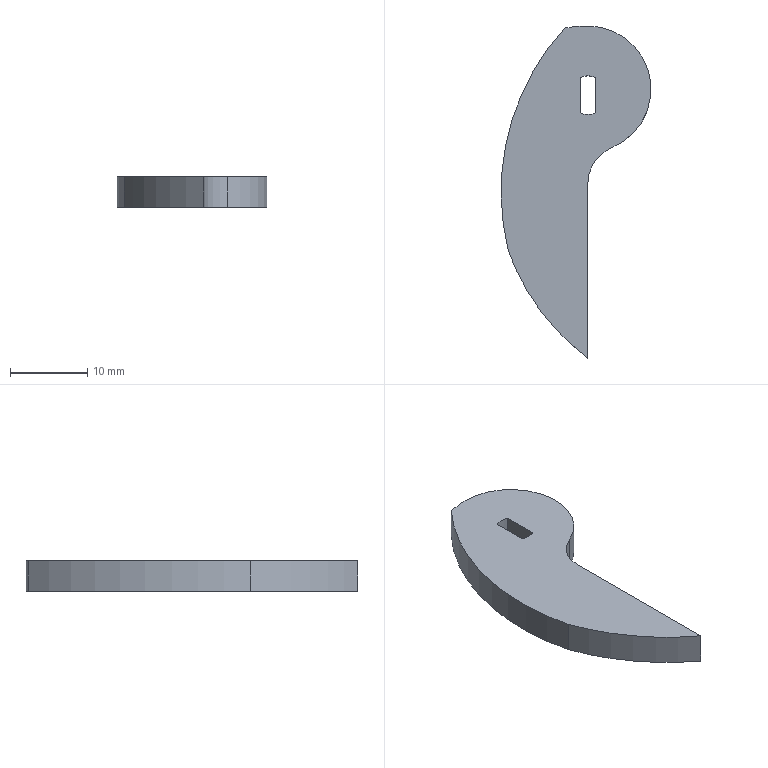Part | SolidWorks | features ICE 4, MirrorStock 1 | 1 solid | 12 faces | box 19.397 x 42.95 x 4 mm | volume 1803 mm3 | cylinder 7 | plane 5 | commonest cylinder face diameters 5 x2 10 x1 16.35 x1 32.7 x1 59.676 x1 62.992 x1
STEP:
#1=CARTESIAN_POINT('',(1.,0.9587,-4.));
#2=VERTEX_POINT('',#1);
#3=CARTESIAN_POINT('',(-1.,0.9587,-4.));
#4=VERTEX_POINT('',#3);
#5=CARTESIAN_POINT('',(0.,3.25,-4.));
#6=DIRECTION('',(0.,0.,-1.));
#7=DIRECTION('',(-1.,0.,0.));
#8=AXIS2_PLACEMENT_3D('',#5,#6,#7);
#9=CIRCLE('',#8,2.5);
#10=EDGE_CURVE('',#2,#4,#9,.T.);
#11=ORIENTED_EDGE('',*,*,#10,.F.);
#12=CARTESIAN_POINT('',(1.,5.541,-4.));
#13=VERTEX_POINT('',#12);
#14=CARTESIAN_POINT('',(1.,4.025,-4.));
#15=DIRECTION('',(0.,-1.,0.));
#16=VECTOR('',#15,1000.);
#17=LINE('',#14,#16);
#18=EDGE_CURVE('',#13,#2,#17,.T.);
#19=ORIENTED_EDGE('',*,*,#18,.F.);
#20=CARTESIAN_POINT('',(-1.,5.541,-4.));
#21=VERTEX_POINT('',#20);
#22=CARTESIAN_POINT('',(0.,3.25,-4.));
#23=DIRECTION('',(0.,0.,-1.));
#24=DIRECTION('',(-1.,0.,0.));
#25=AXIS2_PLACEMENT_3D('',#22,#23,#24);
#26=CIRCLE('',#25,2.5);
#27=EDGE_CURVE('',#21,#13,#26,.T.);
#28=ORIENTED_EDGE('',*,*,#27,.F.);
#29=CARTESIAN_POINT('',(-1.,4.025,-4.));
#30=DIRECTION('',(0.,1.,0.));
#31=VECTOR('',#30,1000.);
#32=LINE('',#29,#31);
#33=EDGE_CURVE('',#4,#21,#32,.T.);
#34=ORIENTED_EDGE('',*,*,#33,.F.);
#35=EDGE_LOOP('',(#11,#19,#28,#34));
#36=FACE_BOUND('',#35,.T.);
#37=CARTESIAN_POINT('',(-3.009,11.921,-4.));
#38=VERTEX_POINT('',#37);
#39=CARTESIAN_POINT('',(-10.302,-16.846,-4.));
#40=VERTEX_POINT('',#39);
#41=CARTESIAN_POINT('',(20.274,-9.29,-4.));
#42=DIRECTION('',(0.,0.,1.));
#43=DIRECTION('',(-1.,0.,0.));
#44=AXIS2_PLACEMENT_3D('',#41,#42,#43);
#45=CIRCLE('',#44,31.496);
#46=EDGE_CURVE('',#38,#40,#45,.T.);
#47=ORIENTED_EDGE('',*,*,#46,.F.);
#48=CARTESIAN_POINT('',(0.,12.2,-4.));
#49=VERTEX_POINT('',#48);
#50=CARTESIAN_POINT('',(0.,-4.15,-4.));
#51=DIRECTION('',(0.,0.,1.));
#52=DIRECTION('',(1.,0.,0.));
#53=AXIS2_PLACEMENT_3D('',#50,#51,#52);
#54=CIRCLE('',#53,16.35);
#55=EDGE_CURVE('',#49,#38,#54,.T.);
#56=ORIENTED_EDGE('',*,*,#55,.F.);
#57=CARTESIAN_POINT('',(3.102,-3.538,-4.));
#58=VERTEX_POINT('',#57);
#59=CARTESIAN_POINT('',(0.,4.025,-4.));
#60=DIRECTION('',(0.,0.,1.));
#61=DIRECTION('',(1.,0.,0.));
#62=AXIS2_PLACEMENT_3D('',#59,#60,#61);
#63=CIRCLE('',#62,8.175);
#64=EDGE_CURVE('',#58,#49,#63,.T.);
#65=ORIENTED_EDGE('',*,*,#64,.F.);
#66=CARTESIAN_POINT('',(0.,-8.164,-4.));
#67=VERTEX_POINT('',#66);
#68=CARTESIAN_POINT('',(5.,-8.164,-4.));
#69=DIRECTION('',(0.,0.,1.));
#70=DIRECTION('',(1.,0.,0.));
#71=AXIS2_PLACEMENT_3D('',#68,#69,#70);
#72=CIRCLE('',#71,5.);
#73=EDGE_CURVE('',#58,#67,#72,.T.);
#74=ORIENTED_EDGE('',*,*,#73,.T.);
#75=CARTESIAN_POINT('',(0.,-30.75,-4.));
#76=VERTEX_POINT('',#75);
#77=CARTESIAN_POINT('',(0.,-20.5,-4.));
#78=DIRECTION('',(0.,1.,0.));
#79=VECTOR('',#78,1000.);
#80=LINE('',#77,#79);
#81=EDGE_CURVE('',#76,#67,#80,.T.);
#82=ORIENTED_EDGE('',*,*,#81,.F.);
#83=CARTESIAN_POINT('',(17.793,-6.798,-4.));
#84=DIRECTION('',(0.,0.,-1.));
#85=DIRECTION('',(-1.,0.,0.));
#86=AXIS2_PLACEMENT_3D('',#83,#84,#85);
#87=CIRCLE('',#86,29.838);
#88=EDGE_CURVE('',#76,#40,#87,.T.);
#89=ORIENTED_EDGE('',*,*,#88,.T.);
#90=EDGE_LOOP('',(#47,#56,#65,#74,#82,#89));
#91=FACE_OUTER_BOUND('',#90,.T.);
#92=CARTESIAN_POINT('',(0.,4.025,-4.));
#93=DIRECTION('',(0.,0.,-1.));
#94=DIRECTION('',(1.,0.,0.));
#95=AXIS2_PLACEMENT_3D('',#92,#93,#94);
#96=PLANE('',#95);
#97=ADVANCED_FACE('',(#36,#91),#96,.T.);
#98=CARTESIAN_POINT('',(1.,0.9587,0.));
#99=VERTEX_POINT('',#98);
#100=CARTESIAN_POINT('',(1.,5.541,0.));
#101=VERTEX_POINT('',#100);
#102=CARTESIAN_POINT('',(1.,5.541,0.));
#103=DIRECTION('',(0.,1.,0.));
#104=VECTOR('',#103,1000.);
#105=LINE('',#102,#104);
#106=EDGE_CURVE('',#99,#101,#105,.T.);
#107=ORIENTED_EDGE('',*,*,#106,.F.);
#108=CARTESIAN_POINT('',(-1.,0.9587,0.));
#109=VERTEX_POINT('',#108);
#110=CARTESIAN_POINT('',(0.,3.25,0.));
#111=DIRECTION('',(0.,0.,1.));
#112=DIRECTION('',(1.,0.,0.));
#113=AXIS2_PLACEMENT_3D('',#110,#111,#112);
#114=CIRCLE('',#113,2.5);
#115=EDGE_CURVE('',#109,#99,#114,.T.);
#116=ORIENTED_EDGE('',*,*,#115,.F.);
#117=CARTESIAN_POINT('',(-1.,5.541,0.));
#118=VERTEX_POINT('',#117);
#119=CARTESIAN_POINT('',(-1.,5.541,0.));
#120=DIRECTION('',(0.,-1.,0.));
#121=VECTOR('',#120,1000.);
#122=LINE('',#119,#121);
#123=EDGE_CURVE('',#118,#109,#122,.T.);
#124=ORIENTED_EDGE('',*,*,#123,.F.);
#125=CARTESIAN_POINT('',(0.,3.25,0.));
#126=DIRECTION('',(0.,0.,1.));
#127=DIRECTION('',(1.,0.,0.));
#128=AXIS2_PLACEMENT_3D('',#125,#126,#127);
#129=CIRCLE('',#128,2.5);
#130=EDGE_CURVE('',#101,#118,#129,.T.);
#131=ORIENTED_EDGE('',*,*,#130,.F.);
#132=EDGE_LOOP('',(#107,#116,#124,#131));
#133=FACE_BOUND('',#132,.T.);
#134=CARTESIAN_POINT('',(0.,12.2,0.));
#135=VERTEX_POINT('',#134);
#136=CARTESIAN_POINT('',(-3.009,11.921,0.));
#137=VERTEX_POINT('',#136);
#138=CARTESIAN_POINT('',(0.,-4.15,0.));
#139=DIRECTION('',(0.,0.,1.));
#140=DIRECTION('',(1.,0.,0.));
#141=AXIS2_PLACEMENT_3D('',#138,#139,#140);
#142=CIRCLE('',#141,16.35);
#143=EDGE_CURVE('',#135,#137,#142,.T.);
#144=ORIENTED_EDGE('',*,*,#143,.T.);
#145=CARTESIAN_POINT('',(-10.302,-16.846,0.));
#146=VERTEX_POINT('',#145);
#147=CARTESIAN_POINT('',(20.274,-9.29,0.));
#148=DIRECTION('',(0.,0.,-1.));
#149=DIRECTION('',(-1.,0.,0.));
#150=AXIS2_PLACEMENT_3D('',#147,#148,#149);
#151=CIRCLE('',#150,31.496);
#152=EDGE_CURVE('',#146,#137,#151,.T.);
#153=ORIENTED_EDGE('',*,*,#152,.F.);
#154=CARTESIAN_POINT('',(0.,-30.75,0.));
#155=VERTEX_POINT('',#154);
#156=CARTESIAN_POINT('',(17.793,-6.798,0.));
#157=DIRECTION('',(0.,0.,-1.));
#158=DIRECTION('',(1.,0.,0.));
#159=AXIS2_PLACEMENT_3D('',#156,#157,#158);
#160=CIRCLE('',#159,29.838);
#161=EDGE_CURVE('',#155,#146,#160,.T.);
#162=ORIENTED_EDGE('',*,*,#161,.F.);
#163=CARTESIAN_POINT('',(0.,-8.164,0.));
#164=VERTEX_POINT('',#163);
#165=CARTESIAN_POINT('',(0.,-20.5,0.));
#166=DIRECTION('',(0.,1.,0.));
#167=VECTOR('',#166,1000.);
#168=LINE('',#165,#167);
#169=EDGE_CURVE('',#155,#164,#168,.T.);
#170=ORIENTED_EDGE('',*,*,#169,.T.);
#171=CARTESIAN_POINT('',(3.102,-3.538,0.));
#172=VERTEX_POINT('',#171);
#173=CARTESIAN_POINT('',(5.,-8.164,0.));
#174=DIRECTION('',(0.,0.,-1.));
#175=DIRECTION('',(1.,0.,0.));
#176=AXIS2_PLACEMENT_3D('',#173,#174,#175);
#177=CIRCLE('',#176,5.);
#178=EDGE_CURVE('',#164,#172,#177,.T.);
#179=ORIENTED_EDGE('',*,*,#178,.T.);
#180=CARTESIAN_POINT('',(0.,4.025,0.));
#181=DIRECTION('',(0.,0.,1.));
#182=DIRECTION('',(1.,0.,0.));
#183=AXIS2_PLACEMENT_3D('',#180,#181,#182);
#184=CIRCLE('',#183,8.175);
#185=EDGE_CURVE('',#172,#135,#184,.T.);
#186=ORIENTED_EDGE('',*,*,#185,.T.);
#187=EDGE_LOOP('',(#144,#153,#162,#170,#179,#186));
#188=FACE_OUTER_BOUND('',#187,.T.);
#189=CARTESIAN_POINT('',(0.,4.025,0.));
#190=DIRECTION('',(0.,0.,-1.));
#191=DIRECTION('',(1.,0.,0.));
#192=AXIS2_PLACEMENT_3D('',#189,#190,#191);
#193=PLANE('',#192);
#194=ADVANCED_FACE('',(#133,#188),#193,.F.);
#195=ORIENTED_EDGE('',*,*,#55,.T.);
#196=CARTESIAN_POINT('',(-3.009,11.921,-10.));
#197=DIRECTION('',(0.,0.,1.));
#198=VECTOR('',#197,1000.);
#199=LINE('',#196,#198);
#200=EDGE_CURVE('',#38,#137,#199,.T.);
#201=ORIENTED_EDGE('',*,*,#200,.T.);
#202=ORIENTED_EDGE('',*,*,#143,.F.);
#203=CARTESIAN_POINT('',(0.,12.2,-4.));
#204=DIRECTION('',(0.,0.,1.));
#205=VECTOR('',#204,1000.);
#206=LINE('',#203,#205);
#207=EDGE_CURVE('',#49,#135,#206,.T.);
#208=ORIENTED_EDGE('',*,*,#207,.F.);
#209=EDGE_LOOP('',(#195,#201,#202,#208));
#210=FACE_OUTER_BOUND('',#209,.T.);
#211=CARTESIAN_POINT('',(0.,-4.15,-4.));
#212=DIRECTION('',(0.,0.,1.));
#213=DIRECTION('',(-1.,0.,0.));
#214=AXIS2_PLACEMENT_3D('',#211,#212,#213);
#215=CYLINDRICAL_SURFACE('',#214,16.35);
#216=ADVANCED_FACE('',(#210),#215,.T.);
#217=CARTESIAN_POINT('',(0.,-8.164,-4.));
#218=DIRECTION('',(0.,0.,-1.));
#219=VECTOR('',#218,1000.);
#220=LINE('',#217,#219);
#221=EDGE_CURVE('',#164,#67,#220,.T.);
#222=ORIENTED_EDGE('',*,*,#221,.T.);
#223=ORIENTED_EDGE('',*,*,#73,.F.);
#224=CARTESIAN_POINT('',(3.102,-3.538,-4.));
#225=DIRECTION('',(0.,0.,1.));
#226=VECTOR('',#225,1000.);
#227=LINE('',#224,#226);
#228=EDGE_CURVE('',#58,#172,#227,.T.);
#229=ORIENTED_EDGE('',*,*,#228,.T.);
#230=ORIENTED_EDGE('',*,*,#178,.F.);
#231=EDGE_LOOP('',(#222,#223,#229,#230));
#232=FACE_OUTER_BOUND('',#231,.T.);
#233=CARTESIAN_POINT('',(5.,-8.164,-4.));
#234=DIRECTION('',(0.,0.,1.));
#235=DIRECTION('',(-1.,0.,0.));
#236=AXIS2_PLACEMENT_3D('',#233,#234,#235);
#237=CYLINDRICAL_SURFACE('',#236,5.);
#238=ADVANCED_FACE('',(#232),#237,.F.);
#239=ORIENTED_EDGE('',*,*,#64,.T.);
#240=ORIENTED_EDGE('',*,*,#207,.T.);
#241=ORIENTED_EDGE('',*,*,#185,.F.);
#242=ORIENTED_EDGE('',*,*,#228,.F.);
#243=EDGE_LOOP('',(#239,#240,#241,#242));
#244=FACE_OUTER_BOUND('',#243,.T.);
#245=CARTESIAN_POINT('',(0.,4.025,-4.));
#246=DIRECTION('',(0.,0.,1.));
#247=DIRECTION('',(-1.,0.,0.));
#248=AXIS2_PLACEMENT_3D('',#245,#246,#247);
#249=CYLINDRICAL_SURFACE('',#248,8.175);
#250=ADVANCED_FACE('',(#244),#249,.T.);
#251=ORIENTED_EDGE('',*,*,#169,.F.);
#252=CARTESIAN_POINT('',(0.,-30.75,-21.304));
#253=DIRECTION('',(0.,0.,1.));
#254=VECTOR('',#253,1000.);
#255=LINE('',#252,#254);
#256=EDGE_CURVE('',#76,#155,#255,.T.);
#257=ORIENTED_EDGE('',*,*,#256,.F.);
#258=ORIENTED_EDGE('',*,*,#81,.T.);
#259=ORIENTED_EDGE('',*,*,#221,.F.);
#260=EDGE_LOOP('',(#251,#257,#258,#259));
#261=FACE_OUTER_BOUND('',#260,.T.);
#262=CARTESIAN_POINT('',(0.,-20.5,-4.));
#263=DIRECTION('',(-1.,0.,0.));
#264=DIRECTION('',(0.,0.,-1.));
#265=AXIS2_PLACEMENT_3D('',#262,#263,#264);
#266=PLANE('',#265);
#267=ADVANCED_FACE('',(#261),#266,.F.);
#268=ORIENTED_EDGE('',*,*,#10,.T.);
#269=CARTESIAN_POINT('',(-1.,0.9587,-10.));
#270=DIRECTION('',(0.,0.,1.));
#271=VECTOR('',#270,1000.);
#272=LINE('',#269,#271);
#273=EDGE_CURVE('',#4,#109,#272,.T.);
#274=ORIENTED_EDGE('',*,*,#273,.T.);
#275=ORIENTED_EDGE('',*,*,#115,.T.);
#276=CARTESIAN_POINT('',(1.,0.9587,-10.));
#277=DIRECTION('',(0.,0.,1.));
#278=VECTOR('',#277,1000.);
#279=LINE('',#276,#278);
#280=EDGE_CURVE('',#2,#99,#279,.T.);
#281=ORIENTED_EDGE('',*,*,#280,.F.);
#282=EDGE_LOOP('',(#268,#274,#275,#281));
#283=FACE_OUTER_BOUND('',#282,.T.);
#284=CARTESIAN_POINT('',(0.,3.25,-10.));
#285=DIRECTION('',(0.,0.,1.));
#286=DIRECTION('',(1.,0.,0.));
#287=AXIS2_PLACEMENT_3D('',#284,#285,#286);
#288=CYLINDRICAL_SURFACE('',#287,2.5);
#289=ADVANCED_FACE('',(#283),#288,.F.);
#290=ORIENTED_EDGE('',*,*,#27,.T.);
#291=CARTESIAN_POINT('',(1.,5.541,-10.));
#292=DIRECTION('',(0.,0.,1.));
#293=VECTOR('',#292,1000.);
#294=LINE('',#291,#293);
#295=EDGE_CURVE('',#13,#101,#294,.T.);
#296=ORIENTED_EDGE('',*,*,#295,.T.);
#297=ORIENTED_EDGE('',*,*,#130,.T.);
#298=CARTESIAN_POINT('',(-1.,5.541,-10.));
#299=DIRECTION('',(0.,0.,1.));
#300=VECTOR('',#299,1000.);
#301=LINE('',#298,#300);
#302=EDGE_CURVE('',#21,#118,#301,.T.);
#303=ORIENTED_EDGE('',*,*,#302,.F.);
#304=EDGE_LOOP('',(#290,#296,#297,#303));
#305=FACE_OUTER_BOUND('',#304,.T.);
#306=CARTESIAN_POINT('',(0.,3.25,-10.));
#307=DIRECTION('',(0.,0.,1.));
#308=DIRECTION('',(1.,0.,0.));
#309=AXIS2_PLACEMENT_3D('',#306,#307,#308);
#310=CYLINDRICAL_SURFACE('',#309,2.5);
#311=ADVANCED_FACE('',(#305),#310,.F.);
#312=ORIENTED_EDGE('',*,*,#18,.T.);
#313=ORIENTED_EDGE('',*,*,#280,.T.);
#314=ORIENTED_EDGE('',*,*,#106,.T.);
#315=ORIENTED_EDGE('',*,*,#295,.F.);
#316=EDGE_LOOP('',(#312,#313,#314,#315));
#317=FACE_OUTER_BOUND('',#316,.T.);
#318=CARTESIAN_POINT('',(1.,5.541,-10.));
#319=DIRECTION('',(1.,0.,0.));
#320=DIRECTION('',(0.,0.,-1.));
#321=AXIS2_PLACEMENT_3D('',#318,#319,#320);
#322=PLANE('',#321);
#323=ADVANCED_FACE('',(#317),#322,.F.);
#324=ORIENTED_EDGE('',*,*,#33,.T.);
#325=ORIENTED_EDGE('',*,*,#302,.T.);
#326=ORIENTED_EDGE('',*,*,#123,.T.);
#327=ORIENTED_EDGE('',*,*,#273,.F.);
#328=EDGE_LOOP('',(#324,#325,#326,#327));
#329=FACE_OUTER_BOUND('',#328,.T.);
#330=CARTESIAN_POINT('',(-1.,5.541,-10.));
#331=DIRECTION('',(-1.,0.,0.));
#332=DIRECTION('',(0.,-1.,0.));
#333=AXIS2_PLACEMENT_3D('',#330,#331,#332);
#334=PLANE('',#333);
#335=ADVANCED_FACE('',(#329),#334,.F.);
#336=ORIENTED_EDGE('',*,*,#88,.F.);
#337=ORIENTED_EDGE('',*,*,#256,.T.);
#338=ORIENTED_EDGE('',*,*,#161,.T.);
#339=CARTESIAN_POINT('',(-10.302,-16.846,-21.304));
#340=DIRECTION('',(0.,0.,1.));
#341=VECTOR('',#340,1000.);
#342=LINE('',#339,#341);
#343=EDGE_CURVE('',#40,#146,#342,.T.);
#344=ORIENTED_EDGE('',*,*,#343,.F.);
#345=EDGE_LOOP('',(#336,#337,#338,#344));
#346=FACE_OUTER_BOUND('',#345,.T.);
#347=CARTESIAN_POINT('',(17.793,-6.798,-21.304));
#348=DIRECTION('',(0.,0.,1.));
#349=DIRECTION('',(1.,0.,0.));
#350=AXIS2_PLACEMENT_3D('',#347,#348,#349);
#351=CYLINDRICAL_SURFACE('',#350,29.838);
#352=ADVANCED_FACE('',(#346),#351,.T.);
#353=ORIENTED_EDGE('',*,*,#46,.T.);
#354=ORIENTED_EDGE('',*,*,#343,.T.);
#355=ORIENTED_EDGE('',*,*,#152,.T.);
#356=ORIENTED_EDGE('',*,*,#200,.F.);
#357=EDGE_LOOP('',(#353,#354,#355,#356));
#358=FACE_OUTER_BOUND('',#357,.T.);
#359=CARTESIAN_POINT('',(20.274,-9.29,-10.));
#360=DIRECTION('',(0.,0.,1.));
#361=DIRECTION('',(1.,0.,0.));
#362=AXIS2_PLACEMENT_3D('',#359,#360,#361);
#363=CYLINDRICAL_SURFACE('',#362,31.496);
#364=ADVANCED_FACE('',(#358),#363,.T.);
#365=CLOSED_SHELL('',(#97,#194,#216,#238,#250,#267,#289,#311,#323,#335,#352,#364));
#366=MANIFOLD_SOLID_BREP('',#365);
#367=CARTESIAN_POINT('',(0.,0.,0.));
#368=DIRECTION('',(0.,0.,1.));
#369=DIRECTION('',(1.,0.,0.));
#370=AXIS2_PLACEMENT_3D('',#367,#368,#369);
#371=(LENGTH_UNIT()NAMED_UNIT(*)SI_UNIT(.MILLI.,.METRE.));
#372=UNCERTAINTY_MEASURE_WITH_UNIT(LENGTH_MEASURE(0.00001),#371,'','');
#373=(NAMED_UNIT(*)PLANE_ANGLE_UNIT()SI_UNIT($,.RADIAN.));
#374=(NAMED_UNIT(*)SI_UNIT($,.STERADIAN.)SOLID_ANGLE_UNIT());
#375=(GEOMETRIC_REPRESENTATION_CONTEXT(3)GLOBAL_UNCERTAINTY_ASSIGNED_CONTEXT((#372))GLOBAL_UNIT_ASSIGNED_CONTEXT((#371,#373,#374))REPRESENTATION_CONTEXT('',''));
#376=ADVANCED_BREP_SHAPE_REPRESENTATION('',(#366,#370),#375);